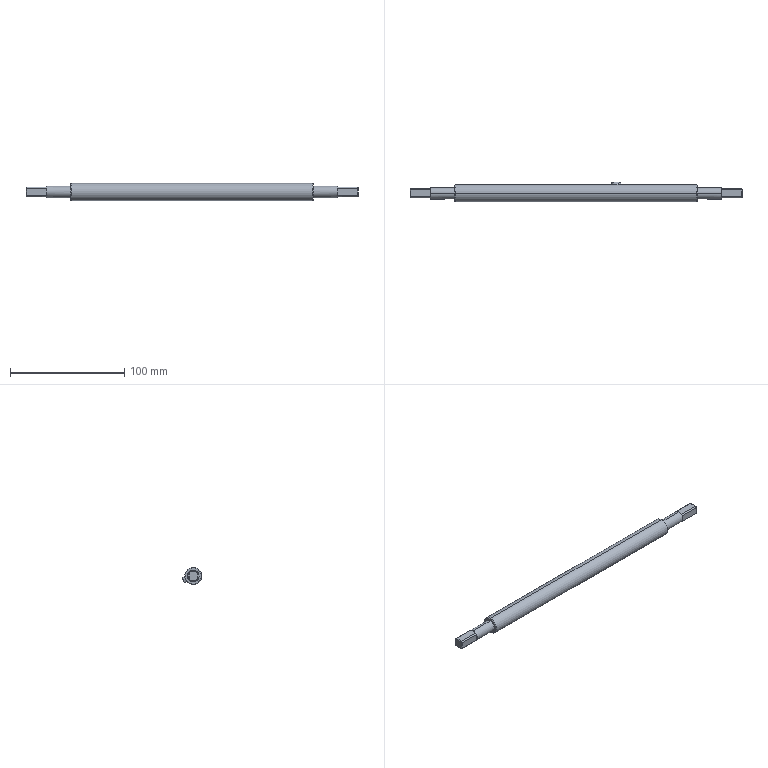Part | SolidWorks | features ICE 3, Chamfer 1, Cut 1, Extrusion 1, Fillet 1, MirrorPattern 1 | 2 solids | 59 faces | box 290 x 17.22 x 15 mm | volume 43056 mm3 | plane 35 | cone 12 | cylinder 12 | commonest cylinder face diameters 5 x6 10 x4 15 x2